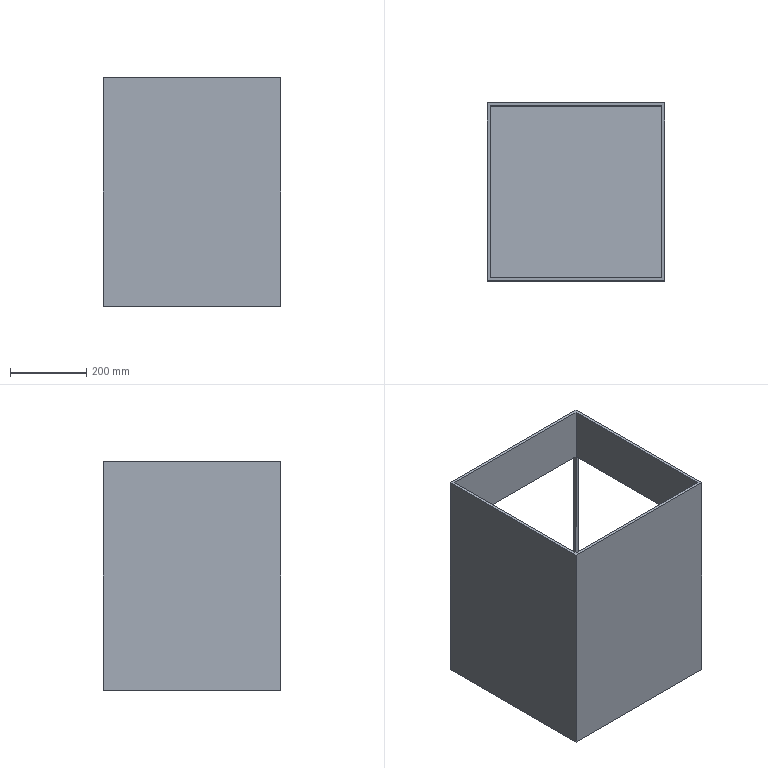Part | SolidWorks | features ICE 3, Extrusion 1 | 1 solid | 15 faces | box 466 x 466 x 600 mm | volume 7173600 mm3 | plane 15
STEP:
#1=CARTESIAN_POINT('',(225.,225.,158.));
#2=VERTEX_POINT('',#1);
#3=CARTESIAN_POINT('',(225.,-225.,158.));
#4=VERTEX_POINT('',#3);
#5=CARTESIAN_POINT('',(225.,225.,158.));
#6=DIRECTION('',(0.,-1.,0.));
#7=VECTOR('',#6,1000.);
#8=LINE('',#5,#7);
#9=EDGE_CURVE('',#2,#4,#8,.T.);
#10=ORIENTED_EDGE('',*,*,#9,.T.);
#11=CARTESIAN_POINT('',(225.,-225.,300.));
#12=VERTEX_POINT('',#11);
#13=CARTESIAN_POINT('',(225.,-225.,300.));
#14=DIRECTION('',(0.,0.,-1.));
#15=VECTOR('',#14,1000.);
#16=LINE('',#13,#15);
#17=EDGE_CURVE('',#12,#4,#16,.T.);
#18=ORIENTED_EDGE('',*,*,#17,.F.);
#19=CARTESIAN_POINT('',(225.,225.,300.));
#20=VERTEX_POINT('',#19);
#21=CARTESIAN_POINT('',(225.,225.,300.));
#22=DIRECTION('',(0.,1.,0.));
#23=VECTOR('',#22,1000.);
#24=LINE('',#21,#23);
#25=EDGE_CURVE('',#12,#20,#24,.T.);
#26=ORIENTED_EDGE('',*,*,#25,.T.);
#27=CARTESIAN_POINT('',(225.,225.,300.));
#28=DIRECTION('',(0.,0.,-1.));
#29=VECTOR('',#28,1000.);
#30=LINE('',#27,#29);
#31=EDGE_CURVE('',#20,#2,#30,.T.);
#32=ORIENTED_EDGE('',*,*,#31,.T.);
#33=EDGE_LOOP('',(#10,#18,#26,#32));
#34=FACE_OUTER_BOUND('',#33,.T.);
#35=CARTESIAN_POINT('',(225.,225.,300.));
#36=DIRECTION('',(-1.,0.,0.));
#37=DIRECTION('',(0.,-1.,0.));
#38=AXIS2_PLACEMENT_3D('',#35,#36,#37);
#39=PLANE('',#38);
#40=ADVANCED_FACE('',(#34),#39,.T.);
#41=CARTESIAN_POINT('',(225.,225.,-292.));
#42=VERTEX_POINT('',#41);
#43=CARTESIAN_POINT('',(225.,225.,-292.));
#44=DIRECTION('',(0.,0.,1.));
#45=VECTOR('',#44,1000.);
#46=LINE('',#43,#45);
#47=EDGE_CURVE('',#42,#2,#46,.T.);
#48=ORIENTED_EDGE('',*,*,#47,.T.);
#49=CARTESIAN_POINT('',(225.,233.,158.));
#50=VERTEX_POINT('',#49);
#51=CARTESIAN_POINT('',(225.,225.,158.));
#52=DIRECTION('',(0.,1.,0.));
#53=VECTOR('',#52,1000.);
#54=LINE('',#51,#53);
#55=EDGE_CURVE('',#2,#50,#54,.T.);
#56=ORIENTED_EDGE('',*,*,#55,.T.);
#57=CARTESIAN_POINT('',(225.,233.,-292.));
#58=VERTEX_POINT('',#57);
#59=CARTESIAN_POINT('',(225.,233.,-292.));
#60=DIRECTION('',(0.,0.,-1.));
#61=VECTOR('',#60,1000.);
#62=LINE('',#59,#61);
#63=EDGE_CURVE('',#50,#58,#62,.T.);
#64=ORIENTED_EDGE('',*,*,#63,.T.);
#65=CARTESIAN_POINT('',(225.,233.,-292.));
#66=DIRECTION('',(0.,-1.,0.));
#67=VECTOR('',#66,1000.);
#68=LINE('',#65,#67);
#69=EDGE_CURVE('',#58,#42,#68,.T.);
#70=ORIENTED_EDGE('',*,*,#69,.T.);
#71=EDGE_LOOP('',(#48,#56,#64,#70));
#72=FACE_OUTER_BOUND('',#71,.T.);
#73=CARTESIAN_POINT('',(225.,225.,300.));
#74=DIRECTION('',(-1.,0.,0.));
#75=DIRECTION('',(0.,-1.,0.));
#76=AXIS2_PLACEMENT_3D('',#73,#74,#75);
#77=PLANE('',#76);
#78=ADVANCED_FACE('',(#72),#77,.T.);
#79=CARTESIAN_POINT('',(-225.,225.,158.));
#80=VERTEX_POINT('',#79);
#81=CARTESIAN_POINT('',(-225.,225.,158.));
#82=DIRECTION('',(1.,0.,0.));
#83=VECTOR('',#82,1000.);
#84=LINE('',#81,#83);
#85=EDGE_CURVE('',#80,#2,#84,.T.);
#86=ORIENTED_EDGE('',*,*,#85,.T.);
#87=ORIENTED_EDGE('',*,*,#31,.F.);
#88=CARTESIAN_POINT('',(-225.,225.,300.));
#89=VERTEX_POINT('',#88);
#90=CARTESIAN_POINT('',(-225.,225.,300.));
#91=DIRECTION('',(-1.,0.,0.));
#92=VECTOR('',#91,1000.);
#93=LINE('',#90,#92);
#94=EDGE_CURVE('',#20,#89,#93,.T.);
#95=ORIENTED_EDGE('',*,*,#94,.T.);
#96=CARTESIAN_POINT('',(-225.,225.,300.));
#97=DIRECTION('',(0.,0.,-1.));
#98=VECTOR('',#97,1000.);
#99=LINE('',#96,#98);
#100=EDGE_CURVE('',#89,#80,#99,.T.);
#101=ORIENTED_EDGE('',*,*,#100,.T.);
#102=EDGE_LOOP('',(#86,#87,#95,#101));
#103=FACE_OUTER_BOUND('',#102,.T.);
#104=CARTESIAN_POINT('',(-225.,225.,300.));
#105=DIRECTION('',(0.,-1.,0.));
#106=DIRECTION('',(0.,0.,-1.));
#107=AXIS2_PLACEMENT_3D('',#104,#105,#106);
#108=PLANE('',#107);
#109=ADVANCED_FACE('',(#103),#108,.T.);
#110=CARTESIAN_POINT('',(-225.,-225.,300.));
#111=VERTEX_POINT('',#110);
#112=CARTESIAN_POINT('',(-225.,-225.,-292.));
#113=VERTEX_POINT('',#112);
#114=CARTESIAN_POINT('',(-225.,-225.,300.));
#115=DIRECTION('',(0.,0.,-1.));
#116=VECTOR('',#115,1000.);
#117=LINE('',#114,#116);
#118=EDGE_CURVE('',#111,#113,#117,.T.);
#119=ORIENTED_EDGE('',*,*,#118,.T.);
#120=CARTESIAN_POINT('',(-225.,233.,-292.));
#121=VERTEX_POINT('',#120);
#122=CARTESIAN_POINT('',(-225.,233.,-292.));
#123=DIRECTION('',(0.,-1.,0.));
#124=VECTOR('',#123,1000.);
#125=LINE('',#122,#124);
#126=EDGE_CURVE('',#121,#113,#125,.T.);
#127=ORIENTED_EDGE('',*,*,#126,.F.);
#128=CARTESIAN_POINT('',(-225.,233.,158.));
#129=VERTEX_POINT('',#128);
#130=CARTESIAN_POINT('',(-225.,233.,-292.));
#131=DIRECTION('',(0.,0.,1.));
#132=VECTOR('',#131,1000.);
#133=LINE('',#130,#132);
#134=EDGE_CURVE('',#121,#129,#133,.T.);
#135=ORIENTED_EDGE('',*,*,#134,.T.);
#136=CARTESIAN_POINT('',(-225.,225.,158.));
#137=DIRECTION('',(0.,1.,0.));
#138=VECTOR('',#137,1000.);
#139=LINE('',#136,#138);
#140=EDGE_CURVE('',#80,#129,#139,.T.);
#141=ORIENTED_EDGE('',*,*,#140,.F.);
#142=ORIENTED_EDGE('',*,*,#100,.F.);
#143=CARTESIAN_POINT('',(-225.,225.,300.));
#144=DIRECTION('',(0.,-1.,0.));
#145=VECTOR('',#144,1000.);
#146=LINE('',#143,#145);
#147=EDGE_CURVE('',#89,#111,#146,.T.);
#148=ORIENTED_EDGE('',*,*,#147,.T.);
#149=EDGE_LOOP('',(#119,#127,#135,#141,#142,#148));
#150=FACE_OUTER_BOUND('',#149,.T.);
#151=CARTESIAN_POINT('',(-225.,225.,300.));
#152=DIRECTION('',(1.,0.,0.));
#153=DIRECTION('',(0.,1.,0.));
#154=AXIS2_PLACEMENT_3D('',#151,#152,#153);
#155=PLANE('',#154);
#156=ADVANCED_FACE('',(#150),#155,.T.);
#157=ORIENTED_EDGE('',*,*,#17,.T.);
#158=CARTESIAN_POINT('',(233.,-225.,158.));
#159=VERTEX_POINT('',#158);
#160=CARTESIAN_POINT('',(225.,-225.,158.));
#161=DIRECTION('',(1.,0.,0.));
#162=VECTOR('',#161,1000.);
#163=LINE('',#160,#162);
#164=EDGE_CURVE('',#4,#159,#163,.T.);
#165=ORIENTED_EDGE('',*,*,#164,.T.);
#166=CARTESIAN_POINT('',(233.,-225.,-292.));
#167=VERTEX_POINT('',#166);
#168=CARTESIAN_POINT('',(233.,-225.,-292.));
#169=DIRECTION('',(0.,0.,-1.));
#170=VECTOR('',#169,1000.);
#171=LINE('',#168,#170);
#172=EDGE_CURVE('',#159,#167,#171,.T.);
#173=ORIENTED_EDGE('',*,*,#172,.T.);
#174=CARTESIAN_POINT('',(-225.,-225.,-292.));
#175=DIRECTION('',(-1.,0.,0.));
#176=VECTOR('',#175,1000.);
#177=LINE('',#174,#176);
#178=EDGE_CURVE('',#167,#113,#177,.T.);
#179=ORIENTED_EDGE('',*,*,#178,.T.);
#180=ORIENTED_EDGE('',*,*,#118,.F.);
#181=CARTESIAN_POINT('',(-225.,-225.,300.));
#182=DIRECTION('',(1.,0.,0.));
#183=VECTOR('',#182,1000.);
#184=LINE('',#181,#183);
#185=EDGE_CURVE('',#111,#12,#184,.T.);
#186=ORIENTED_EDGE('',*,*,#185,.T.);
#187=EDGE_LOOP('',(#157,#165,#173,#179,#180,#186));
#188=FACE_OUTER_BOUND('',#187,.T.);
#189=CARTESIAN_POINT('',(-225.,-225.,300.));
#190=DIRECTION('',(0.,1.,0.));
#191=DIRECTION('',(0.,0.,1.));
#192=AXIS2_PLACEMENT_3D('',#189,#190,#191);
#193=PLANE('',#192);
#194=ADVANCED_FACE('',(#188),#193,.T.);
#195=CARTESIAN_POINT('',(233.,-233.,300.));
#196=VERTEX_POINT('',#195);
#197=CARTESIAN_POINT('',(233.,233.,300.));
#198=VERTEX_POINT('',#197);
#199=CARTESIAN_POINT('',(233.,233.,300.));
#200=DIRECTION('',(0.,1.,0.));
#201=VECTOR('',#200,1000.);
#202=LINE('',#199,#201);
#203=EDGE_CURVE('',#196,#198,#202,.T.);
#204=ORIENTED_EDGE('',*,*,#203,.T.);
#205=CARTESIAN_POINT('',(-233.,233.,300.));
#206=VERTEX_POINT('',#205);
#207=CARTESIAN_POINT('',(-233.,233.,300.));
#208=DIRECTION('',(-1.,0.,0.));
#209=VECTOR('',#208,1000.);
#210=LINE('',#207,#209);
#211=EDGE_CURVE('',#198,#206,#210,.T.);
#212=ORIENTED_EDGE('',*,*,#211,.T.);
#213=CARTESIAN_POINT('',(-233.,-233.,300.));
#214=VERTEX_POINT('',#213);
#215=CARTESIAN_POINT('',(-233.,233.,300.));
#216=DIRECTION('',(0.,-1.,0.));
#217=VECTOR('',#216,1000.);
#218=LINE('',#215,#217);
#219=EDGE_CURVE('',#206,#214,#218,.T.);
#220=ORIENTED_EDGE('',*,*,#219,.T.);
#221=CARTESIAN_POINT('',(-233.,-233.,300.));
#222=DIRECTION('',(1.,0.,0.));
#223=VECTOR('',#222,1000.);
#224=LINE('',#221,#223);
#225=EDGE_CURVE('',#214,#196,#224,.T.);
#226=ORIENTED_EDGE('',*,*,#225,.T.);
#227=EDGE_LOOP('',(#204,#212,#220,#226));
#228=FACE_OUTER_BOUND('',#227,.T.);
#229=ORIENTED_EDGE('',*,*,#94,.F.);
#230=ORIENTED_EDGE('',*,*,#25,.F.);
#231=ORIENTED_EDGE('',*,*,#185,.F.);
#232=ORIENTED_EDGE('',*,*,#147,.F.);
#233=EDGE_LOOP('',(#229,#230,#231,#232));
#234=FACE_BOUND('',#233,.T.);
#235=CARTESIAN_POINT('',(0.,0.,300.));
#236=DIRECTION('',(0.,0.,1.));
#237=DIRECTION('',(1.,0.,0.));
#238=AXIS2_PLACEMENT_3D('',#235,#236,#237);
#239=PLANE('',#238);
#240=ADVANCED_FACE('',(#228,#234),#239,.T.);
#241=CARTESIAN_POINT('',(233.,-233.,-300.));
#242=VERTEX_POINT('',#241);
#243=CARTESIAN_POINT('',(233.,233.,-300.));
#244=VERTEX_POINT('',#243);
#245=CARTESIAN_POINT('',(233.,233.,-300.));
#246=DIRECTION('',(0.,1.,0.));
#247=VECTOR('',#246,1000.);
#248=LINE('',#245,#247);
#249=EDGE_CURVE('',#242,#244,#248,.T.);
#250=ORIENTED_EDGE('',*,*,#249,.F.);
#251=CARTESIAN_POINT('',(-233.,-233.,-300.));
#252=VERTEX_POINT('',#251);
#253=CARTESIAN_POINT('',(-233.,-233.,-300.));
#254=DIRECTION('',(1.,0.,0.));
#255=VECTOR('',#254,1000.);
#256=LINE('',#253,#255);
#257=EDGE_CURVE('',#252,#242,#256,.T.);
#258=ORIENTED_EDGE('',*,*,#257,.F.);
#259=CARTESIAN_POINT('',(-233.,233.,-300.));
#260=VERTEX_POINT('',#259);
#261=CARTESIAN_POINT('',(-233.,233.,-300.));
#262=DIRECTION('',(0.,-1.,0.));
#263=VECTOR('',#262,1000.);
#264=LINE('',#261,#263);
#265=EDGE_CURVE('',#260,#252,#264,.T.);
#266=ORIENTED_EDGE('',*,*,#265,.F.);
#267=CARTESIAN_POINT('',(-233.,233.,-300.));
#268=DIRECTION('',(-1.,0.,0.));
#269=VECTOR('',#268,1000.);
#270=LINE('',#267,#269);
#271=EDGE_CURVE('',#244,#260,#270,.T.);
#272=ORIENTED_EDGE('',*,*,#271,.F.);
#273=EDGE_LOOP('',(#250,#258,#266,#272));
#274=FACE_OUTER_BOUND('',#273,.T.);
#275=CARTESIAN_POINT('',(0.,0.,-300.));
#276=DIRECTION('',(0.,0.,1.));
#277=DIRECTION('',(1.,0.,0.));
#278=AXIS2_PLACEMENT_3D('',#275,#276,#277);
#279=PLANE('',#278);
#280=ADVANCED_FACE('',(#274),#279,.F.);
#281=CARTESIAN_POINT('',(233.,225.,-292.));
#282=VERTEX_POINT('',#281);
#283=CARTESIAN_POINT('',(233.,225.,158.));
#284=VERTEX_POINT('',#283);
#285=CARTESIAN_POINT('',(233.,225.,-292.));
#286=DIRECTION('',(0.,0.,1.));
#287=VECTOR('',#286,1000.);
#288=LINE('',#285,#287);
#289=EDGE_CURVE('',#282,#284,#288,.T.);
#290=ORIENTED_EDGE('',*,*,#289,.F.);
#291=CARTESIAN_POINT('',(233.,225.,-292.));
#292=DIRECTION('',(0.,1.,0.));
#293=VECTOR('',#292,1000.);
#294=LINE('',#291,#293);
#295=EDGE_CURVE('',#167,#282,#294,.T.);
#296=ORIENTED_EDGE('',*,*,#295,.F.);
#297=ORIENTED_EDGE('',*,*,#172,.F.);
#298=CARTESIAN_POINT('',(233.,225.,158.));
#299=DIRECTION('',(0.,-1.,0.));
#300=VECTOR('',#299,1000.);
#301=LINE('',#298,#300);
#302=EDGE_CURVE('',#284,#159,#301,.T.);
#303=ORIENTED_EDGE('',*,*,#302,.F.);
#304=EDGE_LOOP('',(#290,#296,#297,#303));
#305=FACE_BOUND('',#304,.T.);
#306=ORIENTED_EDGE('',*,*,#249,.T.);
#307=CARTESIAN_POINT('',(233.,233.,300.));
#308=DIRECTION('',(0.,0.,-1.));
#309=VECTOR('',#308,1000.);
#310=LINE('',#307,#309);
#311=EDGE_CURVE('',#198,#244,#310,.T.);
#312=ORIENTED_EDGE('',*,*,#311,.F.);
#313=ORIENTED_EDGE('',*,*,#203,.F.);
#314=CARTESIAN_POINT('',(233.,-233.,300.));
#315=DIRECTION('',(0.,0.,-1.));
#316=VECTOR('',#315,1000.);
#317=LINE('',#314,#316);
#318=EDGE_CURVE('',#196,#242,#317,.T.);
#319=ORIENTED_EDGE('',*,*,#318,.T.);
#320=EDGE_LOOP('',(#306,#312,#313,#319));
#321=FACE_OUTER_BOUND('',#320,.T.);
#322=CARTESIAN_POINT('',(233.,233.,300.));
#323=DIRECTION('',(-1.,0.,0.));
#324=DIRECTION('',(0.,-1.,0.));
#325=AXIS2_PLACEMENT_3D('',#322,#323,#324);
#326=PLANE('',#325);
#327=ADVANCED_FACE('',(#305,#321),#326,.F.);
#328=CARTESIAN_POINT('',(-225.,233.,158.));
#329=DIRECTION('',(1.,0.,0.));
#330=VECTOR('',#329,1000.);
#331=LINE('',#328,#330);
#332=EDGE_CURVE('',#129,#50,#331,.T.);
#333=ORIENTED_EDGE('',*,*,#332,.F.);
#334=ORIENTED_EDGE('',*,*,#134,.F.);
#335=CARTESIAN_POINT('',(-225.,233.,-292.));
#336=DIRECTION('',(-1.,0.,0.));
#337=VECTOR('',#336,1000.);
#338=LINE('',#335,#337);
#339=EDGE_CURVE('',#58,#121,#338,.T.);
#340=ORIENTED_EDGE('',*,*,#339,.F.);
#341=ORIENTED_EDGE('',*,*,#63,.F.);
#342=EDGE_LOOP('',(#333,#334,#340,#341));
#343=FACE_BOUND('',#342,.T.);
#344=ORIENTED_EDGE('',*,*,#271,.T.);
#345=CARTESIAN_POINT('',(-233.,233.,300.));
#346=DIRECTION('',(0.,0.,-1.));
#347=VECTOR('',#346,1000.);
#348=LINE('',#345,#347);
#349=EDGE_CURVE('',#206,#260,#348,.T.);
#350=ORIENTED_EDGE('',*,*,#349,.F.);
#351=ORIENTED_EDGE('',*,*,#211,.F.);
#352=ORIENTED_EDGE('',*,*,#311,.T.);
#353=EDGE_LOOP('',(#344,#350,#351,#352));
#354=FACE_OUTER_BOUND('',#353,.T.);
#355=CARTESIAN_POINT('',(-233.,233.,300.));
#356=DIRECTION('',(0.,-1.,0.));
#357=DIRECTION('',(0.,0.,-1.));
#358=AXIS2_PLACEMENT_3D('',#355,#356,#357);
#359=PLANE('',#358);
#360=ADVANCED_FACE('',(#343,#354),#359,.F.);
#361=ORIENTED_EDGE('',*,*,#265,.T.);
#362=CARTESIAN_POINT('',(-233.,-233.,300.));
#363=DIRECTION('',(0.,0.,-1.));
#364=VECTOR('',#363,1000.);
#365=LINE('',#362,#364);
#366=EDGE_CURVE('',#214,#252,#365,.T.);
#367=ORIENTED_EDGE('',*,*,#366,.F.);
#368=ORIENTED_EDGE('',*,*,#219,.F.);
#369=ORIENTED_EDGE('',*,*,#349,.T.);
#370=EDGE_LOOP('',(#361,#367,#368,#369));
#371=FACE_OUTER_BOUND('',#370,.T.);
#372=CARTESIAN_POINT('',(-233.,233.,300.));
#373=DIRECTION('',(1.,0.,0.));
#374=DIRECTION('',(0.,1.,0.));
#375=AXIS2_PLACEMENT_3D('',#372,#373,#374);
#376=PLANE('',#375);
#377=ADVANCED_FACE('',(#371),#376,.F.);
#378=ORIENTED_EDGE('',*,*,#257,.T.);
#379=ORIENTED_EDGE('',*,*,#318,.F.);
#380=ORIENTED_EDGE('',*,*,#225,.F.);
#381=ORIENTED_EDGE('',*,*,#366,.T.);
#382=EDGE_LOOP('',(#378,#379,#380,#381));
#383=FACE_OUTER_BOUND('',#382,.T.);
#384=CARTESIAN_POINT('',(-233.,-233.,300.));
#385=DIRECTION('',(0.,1.,0.));
#386=DIRECTION('',(0.,0.,1.));
#387=AXIS2_PLACEMENT_3D('',#384,#385,#386);
#388=PLANE('',#387);
#389=ADVANCED_FACE('',(#383),#388,.F.);
#390=ORIENTED_EDGE('',*,*,#69,.F.);
#391=ORIENTED_EDGE('',*,*,#339,.T.);
#392=ORIENTED_EDGE('',*,*,#126,.T.);
#393=ORIENTED_EDGE('',*,*,#178,.F.);
#394=ORIENTED_EDGE('',*,*,#295,.T.);
#395=CARTESIAN_POINT('',(225.,225.,-292.));
#396=DIRECTION('',(1.,0.,0.));
#397=VECTOR('',#396,1000.);
#398=LINE('',#395,#397);
#399=EDGE_CURVE('',#42,#282,#398,.T.);
#400=ORIENTED_EDGE('',*,*,#399,.F.);
#401=EDGE_LOOP('',(#390,#391,#392,#393,#394,#400));
#402=FACE_OUTER_BOUND('',#401,.T.);
#403=CARTESIAN_POINT('',(225.,233.,-292.));
#404=DIRECTION('',(0.,0.,-1.));
#405=DIRECTION('',(0.,1.,0.));
#406=AXIS2_PLACEMENT_3D('',#403,#404,#405);
#407=PLANE('',#406);
#408=ADVANCED_FACE('',(#402),#407,.F.);
#409=ORIENTED_EDGE('',*,*,#332,.T.);
#410=ORIENTED_EDGE('',*,*,#55,.F.);
#411=ORIENTED_EDGE('',*,*,#85,.F.);
#412=ORIENTED_EDGE('',*,*,#140,.T.);
#413=EDGE_LOOP('',(#409,#410,#411,#412));
#414=FACE_OUTER_BOUND('',#413,.T.);
#415=CARTESIAN_POINT('',(-225.,225.,158.));
#416=DIRECTION('',(0.,0.,1.));
#417=DIRECTION('',(1.,0.,0.));
#418=AXIS2_PLACEMENT_3D('',#415,#416,#417);
#419=PLANE('',#418);
#420=ADVANCED_FACE('',(#414),#419,.F.);
#421=ORIENTED_EDGE('',*,*,#302,.T.);
#422=ORIENTED_EDGE('',*,*,#164,.F.);
#423=ORIENTED_EDGE('',*,*,#9,.F.);
#424=CARTESIAN_POINT('',(225.,225.,158.));
#425=DIRECTION('',(1.,0.,0.));
#426=VECTOR('',#425,1000.);
#427=LINE('',#424,#426);
#428=EDGE_CURVE('',#2,#284,#427,.T.);
#429=ORIENTED_EDGE('',*,*,#428,.T.);
#430=EDGE_LOOP('',(#421,#422,#423,#429));
#431=FACE_OUTER_BOUND('',#430,.T.);
#432=CARTESIAN_POINT('',(225.,225.,158.));
#433=DIRECTION('',(0.,0.,1.));
#434=DIRECTION('',(0.,-1.,0.));
#435=AXIS2_PLACEMENT_3D('',#432,#433,#434);
#436=PLANE('',#435);
#437=ADVANCED_FACE('',(#431),#436,.F.);
#438=ORIENTED_EDGE('',*,*,#289,.T.);
#439=ORIENTED_EDGE('',*,*,#428,.F.);
#440=ORIENTED_EDGE('',*,*,#47,.F.);
#441=ORIENTED_EDGE('',*,*,#399,.T.);
#442=EDGE_LOOP('',(#438,#439,#440,#441));
#443=FACE_OUTER_BOUND('',#442,.T.);
#444=CARTESIAN_POINT('',(225.,225.,-292.));
#445=DIRECTION('',(0.,1.,0.));
#446=DIRECTION('',(0.,0.,1.));
#447=AXIS2_PLACEMENT_3D('',#444,#445,#446);
#448=PLANE('',#447);
#449=ADVANCED_FACE('',(#443),#448,.F.);
#450=CLOSED_SHELL('',(#40,#78,#109,#156,#194,#240,#280,#327,#360,#377,#389,#408,#420,#437,#449));
#451=MANIFOLD_SOLID_BREP('',#450);
#452=CARTESIAN_POINT('',(0.,0.,0.));
#453=DIRECTION('',(0.,0.,1.));
#454=DIRECTION('',(1.,0.,0.));
#455=AXIS2_PLACEMENT_3D('',#452,#453,#454);
#456=(LENGTH_UNIT()NAMED_UNIT(*)SI_UNIT(.MILLI.,.METRE.));
#457=UNCERTAINTY_MEASURE_WITH_UNIT(LENGTH_MEASURE(0.00001),#456,'','');
#458=(NAMED_UNIT(*)PLANE_ANGLE_UNIT()SI_UNIT($,.RADIAN.));
#459=(NAMED_UNIT(*)SI_UNIT($,.STERADIAN.)SOLID_ANGLE_UNIT());
#460=(GEOMETRIC_REPRESENTATION_CONTEXT(3)GLOBAL_UNCERTAINTY_ASSIGNED_CONTEXT((#457))GLOBAL_UNIT_ASSIGNED_CONTEXT((#456,#458,#459))REPRESENTATION_CONTEXT('',''));
#461=ADVANCED_BREP_SHAPE_REPRESENTATION('',(#451,#455),#460);